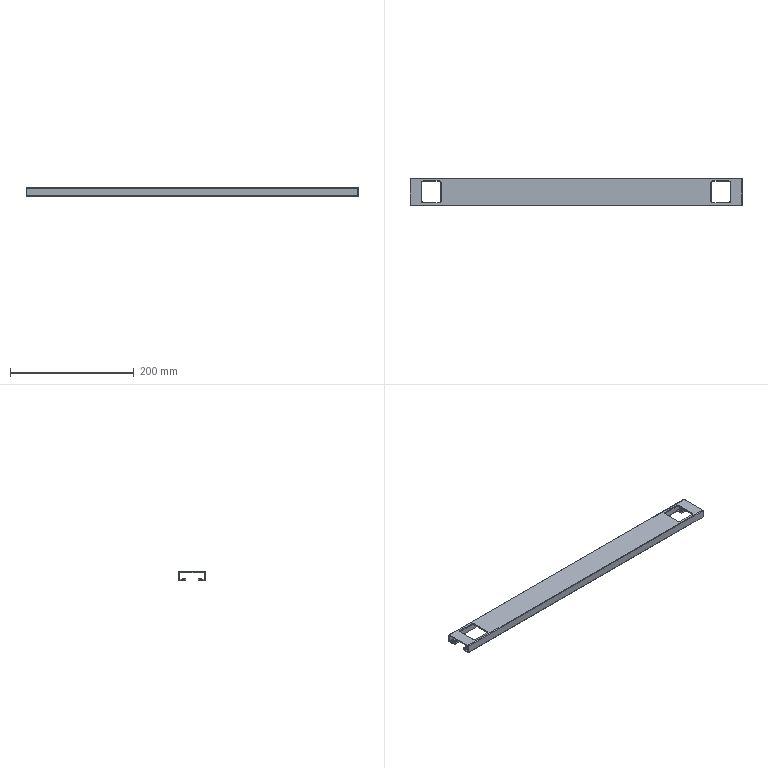Part | NX | features solid 2 | 1 solid | 322 faces | box 537 x 44.3 x 14 mm | volume 88070 mm3 | cylinder 154 | plane 100 | torus 48 | cone 20 | commonest cylinder face diameters 0.2 x48 1 x38 0.6 x36 3.1 x12 4 x8 6 x8